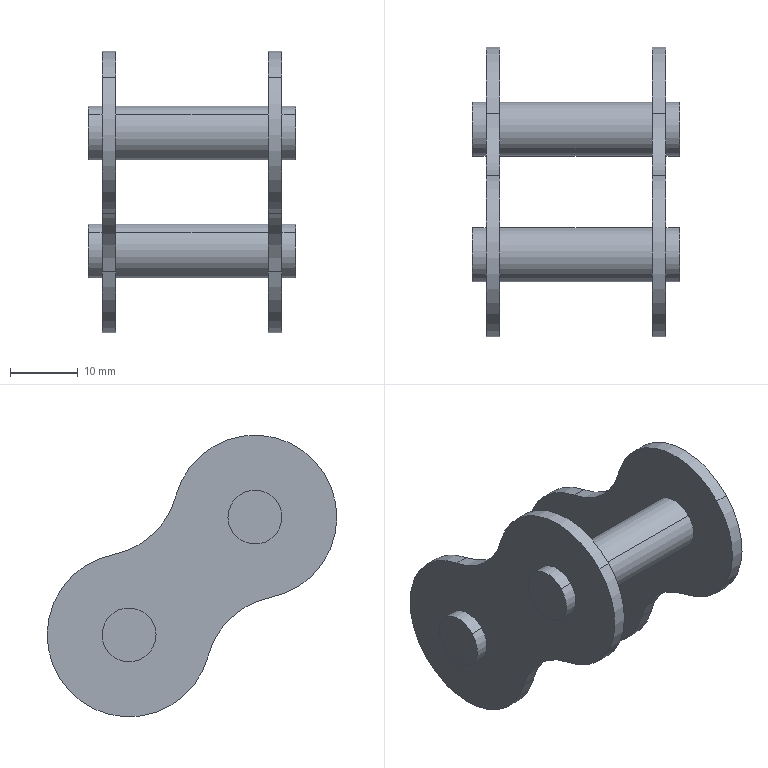Part | STEP file | Mirror 2-38 | 1 solid | 32 faces | box 30.5 x 42.672 x 41.49 mm | volume 6536 mm3 | cylinder 24 | plane 8 | commonest cylinder face diameters 7.94 x12 24.13 x8 23.785 x4
STEP:
#1=CARTESIAN_POINT('',(36.684,-617.915,2791.222));
#2=VERTEX_POINT('',#1);
#3=CARTESIAN_POINT('',(36.684,-624.399,2811.307));
#4=VERTEX_POINT('',#3);
#5=CARTESIAN_POINT('',(36.684,-615.592,2803.061));
#6=DIRECTION('',(-1.,0.,0.));
#7=DIRECTION('',(0.,-0.73,0.6835));
#8=AXIS2_PLACEMENT_3D('',#5,#6,#7);
#9=CIRCLE('',#8,12.065);
#10=EDGE_CURVE('',#2,#4,#9,.T.);
#11=ORIENTED_EDGE('',*,*,#10,.T.);
#12=CARTESIAN_POINT('',(34.684,-624.399,2811.307));
#13=VERTEX_POINT('',#12);
#14=CARTESIAN_POINT('',(36.684,-624.399,2811.307));
#15=DIRECTION('',(-1.,0.,0.));
#16=VECTOR('',#15,1000.);
#17=LINE('',#14,#16);
#18=EDGE_CURVE('',#4,#13,#17,.T.);
#19=ORIENTED_EDGE('',*,*,#18,.T.);
#20=CARTESIAN_POINT('',(34.684,-617.915,2791.222));
#21=VERTEX_POINT('',#20);
#22=CARTESIAN_POINT('',(34.684,-615.592,2803.061));
#23=DIRECTION('',(-1.,0.,0.));
#24=DIRECTION('',(0.,-0.73,0.6835));
#25=AXIS2_PLACEMENT_3D('',#22,#23,#24);
#26=CIRCLE('',#25,12.065);
#27=EDGE_CURVE('',#21,#13,#26,.T.);
#28=ORIENTED_EDGE('',*,*,#27,.F.);
#29=CARTESIAN_POINT('',(36.684,-617.915,2791.222));
#30=DIRECTION('',(-1.,0.,0.));
#31=VECTOR('',#30,1000.);
#32=LINE('',#29,#31);
#33=EDGE_CURVE('',#2,#21,#32,.T.);
#34=ORIENTED_EDGE('',*,*,#33,.F.);
#35=EDGE_LOOP('',(#11,#19,#28,#34));
#36=FACE_OUTER_BOUND('',#35,.T.);
#37=CARTESIAN_POINT('',(36.684,-615.592,2803.061));
#38=DIRECTION('',(-1.,0.,0.));
#39=DIRECTION('',(0.,-0.73,0.6835));
#40=AXIS2_PLACEMENT_3D('',#37,#38,#39);
#41=CYLINDRICAL_SURFACE('',#40,12.065);
#42=ADVANCED_FACE('',(#36),#41,.T.);
#43=CARTESIAN_POINT('',(59.184,-624.399,2811.307));
#44=VERTEX_POINT('',#43);
#45=CARTESIAN_POINT('',(59.184,-603.931,2806.158));
#46=VERTEX_POINT('',#45);
#47=CARTESIAN_POINT('',(59.184,-615.592,2803.061));
#48=DIRECTION('',(-1.,0.,0.));
#49=DIRECTION('',(0.,-0.73,0.6835));
#50=AXIS2_PLACEMENT_3D('',#47,#48,#49);
#51=CIRCLE('',#50,12.065);
#52=EDGE_CURVE('',#44,#46,#51,.T.);
#53=ORIENTED_EDGE('',*,*,#52,.F.);
#54=CARTESIAN_POINT('',(61.184,-624.399,2811.307));
#55=VERTEX_POINT('',#54);
#56=CARTESIAN_POINT('',(59.184,-624.399,2811.307));
#57=DIRECTION('',(1.,0.,0.));
#58=VECTOR('',#57,1000.);
#59=LINE('',#56,#58);
#60=EDGE_CURVE('',#44,#55,#59,.T.);
#61=ORIENTED_EDGE('',*,*,#60,.T.);
#62=CARTESIAN_POINT('',(61.184,-603.931,2806.158));
#63=VERTEX_POINT('',#62);
#64=CARTESIAN_POINT('',(61.184,-615.592,2803.061));
#65=DIRECTION('',(-1.,0.,0.));
#66=DIRECTION('',(0.,-0.73,0.6835));
#67=AXIS2_PLACEMENT_3D('',#64,#65,#66);
#68=CIRCLE('',#67,12.065);
#69=EDGE_CURVE('',#55,#63,#68,.T.);
#70=ORIENTED_EDGE('',*,*,#69,.T.);
#71=CARTESIAN_POINT('',(59.184,-603.931,2806.158));
#72=DIRECTION('',(1.,0.,0.));
#73=VECTOR('',#72,1000.);
#74=LINE('',#71,#73);
#75=EDGE_CURVE('',#46,#63,#74,.T.);
#76=ORIENTED_EDGE('',*,*,#75,.F.);
#77=EDGE_LOOP('',(#53,#61,#70,#76));
#78=FACE_OUTER_BOUND('',#77,.T.);
#79=CARTESIAN_POINT('',(59.184,-615.592,2803.061));
#80=DIRECTION('',(1.,0.,0.));
#81=DIRECTION('',(0.,-0.73,0.6835));
#82=AXIS2_PLACEMENT_3D('',#79,#80,#81);
#83=CYLINDRICAL_SURFACE('',#82,12.065);
#84=ADVANCED_FACE('',(#78),#83,.T.);
#85=CARTESIAN_POINT('',(34.684,-594.152,2782.988));
#86=VERTEX_POINT('',#85);
#87=CARTESIAN_POINT('',(34.684,-599.948,2788.414));
#88=VERTEX_POINT('',#87);
#89=CARTESIAN_POINT('',(34.684,-597.05,2785.701));
#90=DIRECTION('',(-1.,0.,0.));
#91=DIRECTION('',(0.,0.73,-0.6835));
#92=AXIS2_PLACEMENT_3D('',#89,#90,#91);
#93=CIRCLE('',#92,3.97);
#94=EDGE_CURVE('',#86,#88,#93,.T.);
#95=ORIENTED_EDGE('',*,*,#94,.T.);
#96=CARTESIAN_POINT('',(32.684,-599.948,2788.414));
#97=VERTEX_POINT('',#96);
#98=CARTESIAN_POINT('',(47.934,-599.948,2788.414));
#99=DIRECTION('',(1.,0.,0.));
#100=VECTOR('',#99,1000.);
#101=LINE('',#98,#100);
#102=EDGE_CURVE('',#97,#88,#101,.T.);
#103=ORIENTED_EDGE('',*,*,#102,.F.);
#104=CARTESIAN_POINT('',(32.684,-594.152,2782.988));
#105=VERTEX_POINT('',#104);
#106=CARTESIAN_POINT('',(32.684,-597.05,2785.701));
#107=DIRECTION('',(-1.,0.,0.));
#108=DIRECTION('',(0.,-0.73,0.6835));
#109=AXIS2_PLACEMENT_3D('',#106,#107,#108);
#110=CIRCLE('',#109,3.97);
#111=EDGE_CURVE('',#105,#97,#110,.T.);
#112=ORIENTED_EDGE('',*,*,#111,.F.);
#113=CARTESIAN_POINT('',(47.934,-594.152,2782.988));
#114=DIRECTION('',(1.,0.,0.));
#115=VECTOR('',#114,1000.);
#116=LINE('',#113,#115);
#117=EDGE_CURVE('',#105,#86,#116,.T.);
#118=ORIENTED_EDGE('',*,*,#117,.T.);
#119=EDGE_LOOP('',(#95,#103,#112,#118));
#120=FACE_OUTER_BOUND('',#119,.T.);
#121=CARTESIAN_POINT('',(47.934,-597.05,2785.701));
#122=DIRECTION('',(-1.,0.,0.));
#123=DIRECTION('',(0.,-0.73,0.6835));
#124=AXIS2_PLACEMENT_3D('',#121,#122,#123);
#125=CYLINDRICAL_SURFACE('',#124,3.97);
#126=ADVANCED_FACE('',(#120),#125,.T.);
#127=CARTESIAN_POINT('',(34.684,-612.694,2800.348));
#128=VERTEX_POINT('',#127);
#129=CARTESIAN_POINT('',(34.684,-618.49,2805.774));
#130=VERTEX_POINT('',#129);
#131=CARTESIAN_POINT('',(34.684,-615.592,2803.061));
#132=DIRECTION('',(-1.,0.,0.));
#133=DIRECTION('',(0.,0.73,-0.6835));
#134=AXIS2_PLACEMENT_3D('',#131,#132,#133);
#135=CIRCLE('',#134,3.97);
#136=EDGE_CURVE('',#128,#130,#135,.T.);
#137=ORIENTED_EDGE('',*,*,#136,.T.);
#138=CARTESIAN_POINT('',(32.684,-618.49,2805.774));
#139=VERTEX_POINT('',#138);
#140=CARTESIAN_POINT('',(47.934,-618.49,2805.774));
#141=DIRECTION('',(1.,0.,0.));
#142=VECTOR('',#141,1000.);
#143=LINE('',#140,#142);
#144=EDGE_CURVE('',#139,#130,#143,.T.);
#145=ORIENTED_EDGE('',*,*,#144,.F.);
#146=CARTESIAN_POINT('',(32.684,-612.694,2800.348));
#147=VERTEX_POINT('',#146);
#148=CARTESIAN_POINT('',(32.684,-615.592,2803.061));
#149=DIRECTION('',(-1.,0.,0.));
#150=DIRECTION('',(0.,-0.73,0.6835));
#151=AXIS2_PLACEMENT_3D('',#148,#149,#150);
#152=CIRCLE('',#151,3.97);
#153=EDGE_CURVE('',#147,#139,#152,.T.);
#154=ORIENTED_EDGE('',*,*,#153,.F.);
#155=CARTESIAN_POINT('',(47.934,-612.694,2800.348));
#156=DIRECTION('',(1.,0.,0.));
#157=VECTOR('',#156,1000.);
#158=LINE('',#155,#157);
#159=EDGE_CURVE('',#147,#128,#158,.T.);
#160=ORIENTED_EDGE('',*,*,#159,.T.);
#161=EDGE_LOOP('',(#137,#145,#154,#160));
#162=FACE_OUTER_BOUND('',#161,.T.);
#163=CARTESIAN_POINT('',(47.934,-615.592,2803.061));
#164=DIRECTION('',(-1.,0.,0.));
#165=DIRECTION('',(0.,-0.73,0.6835));
#166=AXIS2_PLACEMENT_3D('',#163,#164,#165);
#167=CYLINDRICAL_SURFACE('',#166,3.97);
#168=ADVANCED_FACE('',(#162),#167,.T.);
#169=CARTESIAN_POINT('',(36.684,-594.727,2797.54));
#170=VERTEX_POINT('',#169);
#171=CARTESIAN_POINT('',(36.684,-588.243,2777.455));
#172=VERTEX_POINT('',#171);
#173=CARTESIAN_POINT('',(36.684,-597.05,2785.701));
#174=DIRECTION('',(-1.,0.,0.));
#175=DIRECTION('',(0.,-0.73,0.6835));
#176=AXIS2_PLACEMENT_3D('',#173,#174,#175);
#177=CIRCLE('',#176,12.065);
#178=EDGE_CURVE('',#170,#172,#177,.T.);
#179=ORIENTED_EDGE('',*,*,#178,.T.);
#180=CARTESIAN_POINT('',(34.684,-588.243,2777.455));
#181=VERTEX_POINT('',#180);
#182=CARTESIAN_POINT('',(36.684,-588.243,2777.455));
#183=DIRECTION('',(-1.,0.,0.));
#184=VECTOR('',#183,1000.);
#185=LINE('',#182,#184);
#186=EDGE_CURVE('',#172,#181,#185,.T.);
#187=ORIENTED_EDGE('',*,*,#186,.T.);
#188=CARTESIAN_POINT('',(34.684,-594.727,2797.54));
#189=VERTEX_POINT('',#188);
#190=CARTESIAN_POINT('',(34.684,-597.05,2785.701));
#191=DIRECTION('',(-1.,0.,0.));
#192=DIRECTION('',(0.,-0.73,0.6835));
#193=AXIS2_PLACEMENT_3D('',#190,#191,#192);
#194=CIRCLE('',#193,12.065);
#195=EDGE_CURVE('',#189,#181,#194,.T.);
#196=ORIENTED_EDGE('',*,*,#195,.F.);
#197=CARTESIAN_POINT('',(36.684,-594.727,2797.54));
#198=DIRECTION('',(-1.,0.,0.));
#199=VECTOR('',#198,1000.);
#200=LINE('',#197,#199);
#201=EDGE_CURVE('',#170,#189,#200,.T.);
#202=ORIENTED_EDGE('',*,*,#201,.F.);
#203=EDGE_LOOP('',(#179,#187,#196,#202));
#204=FACE_OUTER_BOUND('',#203,.T.);
#205=CARTESIAN_POINT('',(36.684,-597.05,2785.701));
#206=DIRECTION('',(-1.,0.,0.));
#207=DIRECTION('',(0.,-0.73,0.6835));
#208=AXIS2_PLACEMENT_3D('',#205,#206,#207);
#209=CYLINDRICAL_SURFACE('',#208,12.065);
#210=ADVANCED_FACE('',(#204),#209,.T.);
#211=CARTESIAN_POINT('',(36.684,-599.948,2788.414));
#212=VERTEX_POINT('',#211);
#213=CARTESIAN_POINT('',(36.684,-594.152,2782.988));
#214=VERTEX_POINT('',#213);
#215=CARTESIAN_POINT('',(36.684,-597.05,2785.701));
#216=DIRECTION('',(-1.,0.,0.));
#217=DIRECTION('',(0.,-0.73,0.6835));
#218=AXIS2_PLACEMENT_3D('',#215,#216,#217);
#219=CIRCLE('',#218,3.97);
#220=EDGE_CURVE('',#212,#214,#219,.T.);
#221=ORIENTED_EDGE('',*,*,#220,.F.);
#222=CARTESIAN_POINT('',(59.184,-599.948,2788.414));
#223=VERTEX_POINT('',#222);
#224=CARTESIAN_POINT('',(47.934,-599.948,2788.414));
#225=DIRECTION('',(-1.,0.,0.));
#226=VECTOR('',#225,1000.);
#227=LINE('',#224,#226);
#228=EDGE_CURVE('',#223,#212,#227,.T.);
#229=ORIENTED_EDGE('',*,*,#228,.F.);
#230=CARTESIAN_POINT('',(59.184,-594.152,2782.988));
#231=VERTEX_POINT('',#230);
#232=CARTESIAN_POINT('',(59.184,-597.05,2785.701));
#233=DIRECTION('',(-1.,0.,0.));
#234=DIRECTION('',(0.,-0.73,0.6835));
#235=AXIS2_PLACEMENT_3D('',#232,#233,#234);
#236=CIRCLE('',#235,3.97);
#237=EDGE_CURVE('',#223,#231,#236,.T.);
#238=ORIENTED_EDGE('',*,*,#237,.T.);
#239=CARTESIAN_POINT('',(47.934,-594.152,2782.988));
#240=DIRECTION('',(-1.,0.,0.));
#241=VECTOR('',#240,1000.);
#242=LINE('',#239,#241);
#243=EDGE_CURVE('',#231,#214,#242,.T.);
#244=ORIENTED_EDGE('',*,*,#243,.T.);
#245=EDGE_LOOP('',(#221,#229,#238,#244));
#246=FACE_OUTER_BOUND('',#245,.T.);
#247=CARTESIAN_POINT('',(47.934,-597.05,2785.701));
#248=DIRECTION('',(1.,0.,0.));
#249=DIRECTION('',(0.,-0.73,0.6835));
#250=AXIS2_PLACEMENT_3D('',#247,#248,#249);
#251=CYLINDRICAL_SURFACE('',#250,3.97);
#252=ADVANCED_FACE('',(#246),#251,.T.);
#253=CARTESIAN_POINT('',(61.184,-599.948,2788.414));
#254=VERTEX_POINT('',#253);
#255=CARTESIAN_POINT('',(61.184,-594.152,2782.988));
#256=VERTEX_POINT('',#255);
#257=CARTESIAN_POINT('',(61.184,-597.05,2785.701));
#258=DIRECTION('',(-1.,0.,0.));
#259=DIRECTION('',(0.,0.73,-0.6835));
#260=AXIS2_PLACEMENT_3D('',#257,#258,#259);
#261=CIRCLE('',#260,3.97);
#262=EDGE_CURVE('',#254,#256,#261,.T.);
#263=ORIENTED_EDGE('',*,*,#262,.F.);
#264=CARTESIAN_POINT('',(63.184,-599.948,2788.414));
#265=VERTEX_POINT('',#264);
#266=CARTESIAN_POINT('',(47.934,-599.948,2788.414));
#267=DIRECTION('',(-1.,0.,0.));
#268=VECTOR('',#267,1000.);
#269=LINE('',#266,#268);
#270=EDGE_CURVE('',#265,#254,#269,.T.);
#271=ORIENTED_EDGE('',*,*,#270,.F.);
#272=CARTESIAN_POINT('',(63.184,-594.152,2782.988));
#273=VERTEX_POINT('',#272);
#274=CARTESIAN_POINT('',(63.184,-597.05,2785.701));
#275=DIRECTION('',(-1.,0.,0.));
#276=DIRECTION('',(0.,-0.73,0.6835));
#277=AXIS2_PLACEMENT_3D('',#274,#275,#276);
#278=CIRCLE('',#277,3.97);
#279=EDGE_CURVE('',#265,#273,#278,.T.);
#280=ORIENTED_EDGE('',*,*,#279,.T.);
#281=CARTESIAN_POINT('',(47.934,-594.152,2782.988));
#282=DIRECTION('',(-1.,0.,0.));
#283=VECTOR('',#282,1000.);
#284=LINE('',#281,#283);
#285=EDGE_CURVE('',#273,#256,#284,.T.);
#286=ORIENTED_EDGE('',*,*,#285,.T.);
#287=EDGE_LOOP('',(#263,#271,#280,#286));
#288=FACE_OUTER_BOUND('',#287,.T.);
#289=CARTESIAN_POINT('',(47.934,-597.05,2785.701));
#290=DIRECTION('',(1.,0.,0.));
#291=DIRECTION('',(0.,-0.73,0.6835));
#292=AXIS2_PLACEMENT_3D('',#289,#290,#291);
#293=CYLINDRICAL_SURFACE('',#292,3.97);
#294=ADVANCED_FACE('',(#288),#293,.T.);
#295=CARTESIAN_POINT('',(36.684,-618.49,2805.774));
#296=VERTEX_POINT('',#295);
#297=CARTESIAN_POINT('',(36.684,-612.694,2800.348));
#298=VERTEX_POINT('',#297);
#299=CARTESIAN_POINT('',(36.684,-615.592,2803.061));
#300=DIRECTION('',(-1.,0.,0.));
#301=DIRECTION('',(0.,-0.73,0.6835));
#302=AXIS2_PLACEMENT_3D('',#299,#300,#301);
#303=CIRCLE('',#302,3.97);
#304=EDGE_CURVE('',#296,#298,#303,.T.);
#305=ORIENTED_EDGE('',*,*,#304,.F.);
#306=CARTESIAN_POINT('',(59.184,-618.49,2805.774));
#307=VERTEX_POINT('',#306);
#308=CARTESIAN_POINT('',(47.934,-618.49,2805.774));
#309=DIRECTION('',(-1.,0.,0.));
#310=VECTOR('',#309,1000.);
#311=LINE('',#308,#310);
#312=EDGE_CURVE('',#307,#296,#311,.T.);
#313=ORIENTED_EDGE('',*,*,#312,.F.);
#314=CARTESIAN_POINT('',(59.184,-612.694,2800.348));
#315=VERTEX_POINT('',#314);
#316=CARTESIAN_POINT('',(59.184,-615.592,2803.061));
#317=DIRECTION('',(-1.,0.,0.));
#318=DIRECTION('',(0.,-0.73,0.6835));
#319=AXIS2_PLACEMENT_3D('',#316,#317,#318);
#320=CIRCLE('',#319,3.97);
#321=EDGE_CURVE('',#307,#315,#320,.T.);
#322=ORIENTED_EDGE('',*,*,#321,.T.);
#323=CARTESIAN_POINT('',(47.934,-612.694,2800.348));
#324=DIRECTION('',(-1.,0.,0.));
#325=VECTOR('',#324,1000.);
#326=LINE('',#323,#325);
#327=EDGE_CURVE('',#315,#298,#326,.T.);
#328=ORIENTED_EDGE('',*,*,#327,.T.);
#329=EDGE_LOOP('',(#305,#313,#322,#328));
#330=FACE_OUTER_BOUND('',#329,.T.);
#331=CARTESIAN_POINT('',(47.934,-615.592,2803.061));
#332=DIRECTION('',(1.,0.,0.));
#333=DIRECTION('',(0.,-0.73,0.6835));
#334=AXIS2_PLACEMENT_3D('',#331,#332,#333);
#335=CYLINDRICAL_SURFACE('',#334,3.97);
#336=ADVANCED_FACE('',(#330),#335,.T.);
#337=CARTESIAN_POINT('',(61.184,-618.49,2805.774));
#338=VERTEX_POINT('',#337);
#339=CARTESIAN_POINT('',(61.184,-612.694,2800.348));
#340=VERTEX_POINT('',#339);
#341=CARTESIAN_POINT('',(61.184,-615.592,2803.061));
#342=DIRECTION('',(-1.,0.,0.));
#343=DIRECTION('',(0.,0.73,-0.6835));
#344=AXIS2_PLACEMENT_3D('',#341,#342,#343);
#345=CIRCLE('',#344,3.97);
#346=EDGE_CURVE('',#338,#340,#345,.T.);
#347=ORIENTED_EDGE('',*,*,#346,.F.);
#348=CARTESIAN_POINT('',(63.184,-618.49,2805.774));
#349=VERTEX_POINT('',#348);
#350=CARTESIAN_POINT('',(47.934,-618.49,2805.774));
#351=DIRECTION('',(-1.,0.,0.));
#352=VECTOR('',#351,1000.);
#353=LINE('',#350,#352);
#354=EDGE_CURVE('',#349,#338,#353,.T.);
#355=ORIENTED_EDGE('',*,*,#354,.F.);
#356=CARTESIAN_POINT('',(63.184,-612.694,2800.348));
#357=VERTEX_POINT('',#356);
#358=CARTESIAN_POINT('',(63.184,-615.592,2803.061));
#359=DIRECTION('',(-1.,0.,0.));
#360=DIRECTION('',(0.,-0.73,0.6835));
#361=AXIS2_PLACEMENT_3D('',#358,#359,#360);
#362=CIRCLE('',#361,3.97);
#363=EDGE_CURVE('',#349,#357,#362,.T.);
#364=ORIENTED_EDGE('',*,*,#363,.T.);
#365=CARTESIAN_POINT('',(47.934,-612.694,2800.348));
#366=DIRECTION('',(-1.,0.,0.));
#367=VECTOR('',#366,1000.);
#368=LINE('',#365,#367);
#369=EDGE_CURVE('',#357,#340,#368,.T.);
#370=ORIENTED_EDGE('',*,*,#369,.T.);
#371=EDGE_LOOP('',(#347,#355,#364,#370));
#372=FACE_OUTER_BOUND('',#371,.T.);
#373=CARTESIAN_POINT('',(47.934,-615.592,2803.061));
#374=DIRECTION('',(1.,0.,0.));
#375=DIRECTION('',(0.,-0.73,0.6835));
#376=AXIS2_PLACEMENT_3D('',#373,#374,#375);
#377=CYLINDRICAL_SURFACE('',#376,3.97);
#378=ADVANCED_FACE('',(#372),#377,.T.);
#379=CARTESIAN_POINT('',(59.184,-588.243,2777.455));
#380=VERTEX_POINT('',#379);
#381=CARTESIAN_POINT('',(59.184,-608.711,2782.604));
#382=VERTEX_POINT('',#381);
#383=CARTESIAN_POINT('',(59.184,-597.05,2785.701));
#384=DIRECTION('',(-1.,0.,0.));
#385=DIRECTION('',(0.,-0.73,0.6835));
#386=AXIS2_PLACEMENT_3D('',#383,#384,#385);
#387=CIRCLE('',#386,12.065);
#388=EDGE_CURVE('',#380,#382,#387,.T.);
#389=ORIENTED_EDGE('',*,*,#388,.F.);
#390=CARTESIAN_POINT('',(61.184,-588.243,2777.455));
#391=VERTEX_POINT('',#390);
#392=CARTESIAN_POINT('',(59.184,-588.243,2777.455));
#393=DIRECTION('',(1.,0.,0.));
#394=VECTOR('',#393,1000.);
#395=LINE('',#392,#394);
#396=EDGE_CURVE('',#380,#391,#395,.T.);
#397=ORIENTED_EDGE('',*,*,#396,.T.);
#398=CARTESIAN_POINT('',(61.184,-608.711,2782.604));
#399=VERTEX_POINT('',#398);
#400=CARTESIAN_POINT('',(61.184,-597.05,2785.701));
#401=DIRECTION('',(-1.,0.,0.));
#402=DIRECTION('',(0.,-0.73,0.6835));
#403=AXIS2_PLACEMENT_3D('',#400,#401,#402);
#404=CIRCLE('',#403,12.065);
#405=EDGE_CURVE('',#391,#399,#404,.T.);
#406=ORIENTED_EDGE('',*,*,#405,.T.);
#407=CARTESIAN_POINT('',(59.184,-608.711,2782.604));
#408=DIRECTION('',(1.,0.,0.));
#409=VECTOR('',#408,1000.);
#410=LINE('',#407,#409);
#411=EDGE_CURVE('',#382,#399,#410,.T.);
#412=ORIENTED_EDGE('',*,*,#411,.F.);
#413=EDGE_LOOP('',(#389,#397,#406,#412));
#414=FACE_OUTER_BOUND('',#413,.T.);
#415=CARTESIAN_POINT('',(59.184,-597.05,2785.701));
#416=DIRECTION('',(1.,0.,0.));
#417=DIRECTION('',(0.,-0.73,0.6835));
#418=AXIS2_PLACEMENT_3D('',#415,#416,#417);
#419=CYLINDRICAL_SURFACE('',#418,12.065);
#420=ADVANCED_FACE('',(#414),#419,.T.);
#421=CARTESIAN_POINT('',(59.184,-594.727,2797.54));
#422=VERTEX_POINT('',#421);
#423=CARTESIAN_POINT('',(59.184,-592.437,2809.21));
#424=DIRECTION('',(1.,0.,0.));
#425=DIRECTION('',(0.,0.73,-0.6835));
#426=AXIS2_PLACEMENT_3D('',#423,#424,#425);
#427=CIRCLE('',#426,11.892);
#428=EDGE_CURVE('',#46,#422,#427,.T.);
#429=ORIENTED_EDGE('',*,*,#428,.T.);
#430=CARTESIAN_POINT('',(59.184,-597.05,2785.701));
#431=DIRECTION('',(-1.,0.,0.));
#432=DIRECTION('',(0.,-0.73,0.6835));
#433=AXIS2_PLACEMENT_3D('',#430,#431,#432);
#434=CIRCLE('',#433,12.065);
#435=EDGE_CURVE('',#422,#380,#434,.T.);
#436=ORIENTED_EDGE('',*,*,#435,.T.);
#437=ORIENTED_EDGE('',*,*,#388,.T.);
#438=CARTESIAN_POINT('',(59.184,-617.915,2791.222));
#439=VERTEX_POINT('',#438);
#440=CARTESIAN_POINT('',(59.184,-620.205,2779.552));
#441=DIRECTION('',(1.,0.,0.));
#442=DIRECTION('',(0.,-0.73,0.6835));
#443=AXIS2_PLACEMENT_3D('',#440,#441,#442);
#444=CIRCLE('',#443,11.892);
#445=EDGE_CURVE('',#382,#439,#444,.T.);
#446=ORIENTED_EDGE('',*,*,#445,.T.);
#447=CARTESIAN_POINT('',(59.184,-615.592,2803.061));
#448=DIRECTION('',(-1.,0.,0.));
#449=DIRECTION('',(0.,-0.73,0.6835));
#450=AXIS2_PLACEMENT_3D('',#447,#448,#449);
#451=CIRCLE('',#450,12.065);
#452=EDGE_CURVE('',#439,#44,#451,.T.);
#453=ORIENTED_EDGE('',*,*,#452,.T.);
#454=ORIENTED_EDGE('',*,*,#52,.T.);
#455=EDGE_LOOP('',(#429,#436,#437,#446,#453,#454));
#456=FACE_OUTER_BOUND('',#455,.T.);
#457=CARTESIAN_POINT('',(59.184,-615.592,2803.061));
#458=DIRECTION('',(-1.,0.,0.));
#459=DIRECTION('',(0.,-0.73,0.6835));
#460=AXIS2_PLACEMENT_3D('',#457,#458,#459);
#461=CIRCLE('',#460,3.97);
#462=EDGE_CURVE('',#315,#307,#461,.T.);
#463=ORIENTED_EDGE('',*,*,#462,.F.);
#464=ORIENTED_EDGE('',*,*,#321,.F.);
#465=EDGE_LOOP('',(#463,#464));
#466=FACE_BOUND('',#465,.T.);
#467=CARTESIAN_POINT('',(59.184,-597.05,2785.701));
#468=DIRECTION('',(-1.,0.,0.));
#469=DIRECTION('',(0.,-0.73,0.6835));
#470=AXIS2_PLACEMENT_3D('',#467,#468,#469);
#471=CIRCLE('',#470,3.97);
#472=EDGE_CURVE('',#231,#223,#471,.T.);
#473=ORIENTED_EDGE('',*,*,#472,.F.);
#474=ORIENTED_EDGE('',*,*,#237,.F.);
#475=EDGE_LOOP('',(#473,#474));
#476=FACE_BOUND('',#475,.T.);
#477=CARTESIAN_POINT('',(59.184,-594.743,2797.456));
#478=DIRECTION('',(1.,0.,0.));
#479=DIRECTION('',(0.,-0.73,0.6835));
#480=AXIS2_PLACEMENT_3D('',#477,#478,#479);
#481=PLANE('',#480);
#482=ADVANCED_FACE('',(#456,#466,#476),#481,.F.);
#483=CARTESIAN_POINT('',(61.184,-615.592,2803.061));
#484=DIRECTION('',(-1.,0.,0.));
#485=DIRECTION('',(0.,0.73,-0.6835));
#486=AXIS2_PLACEMENT_3D('',#483,#484,#485);
#487=CIRCLE('',#486,3.97);
#488=EDGE_CURVE('',#340,#338,#487,.T.);
#489=ORIENTED_EDGE('',*,*,#488,.T.);
#490=ORIENTED_EDGE('',*,*,#346,.T.);
#491=EDGE_LOOP('',(#489,#490));
#492=FACE_BOUND('',#491,.T.);
#493=CARTESIAN_POINT('',(61.184,-594.727,2797.54));
#494=VERTEX_POINT('',#493);
#495=CARTESIAN_POINT('',(61.184,-592.437,2809.21));
#496=DIRECTION('',(1.,0.,0.));
#497=DIRECTION('',(0.,0.73,-0.6835));
#498=AXIS2_PLACEMENT_3D('',#495,#496,#497);
#499=CIRCLE('',#498,11.892);
#500=EDGE_CURVE('',#63,#494,#499,.T.);
#501=ORIENTED_EDGE('',*,*,#500,.F.);
#502=ORIENTED_EDGE('',*,*,#69,.F.);
#503=CARTESIAN_POINT('',(61.184,-617.915,2791.222));
#504=VERTEX_POINT('',#503);
#505=CARTESIAN_POINT('',(61.184,-615.592,2803.061));
#506=DIRECTION('',(-1.,0.,0.));
#507=DIRECTION('',(0.,-0.73,0.6835));
#508=AXIS2_PLACEMENT_3D('',#505,#506,#507);
#509=CIRCLE('',#508,12.065);
#510=EDGE_CURVE('',#504,#55,#509,.T.);
#511=ORIENTED_EDGE('',*,*,#510,.F.);
#512=CARTESIAN_POINT('',(61.184,-620.205,2779.552));
#513=DIRECTION('',(1.,0.,0.));
#514=DIRECTION('',(0.,-0.73,0.6835));
#515=AXIS2_PLACEMENT_3D('',#512,#513,#514);
#516=CIRCLE('',#515,11.892);
#517=EDGE_CURVE('',#399,#504,#516,.T.);
#518=ORIENTED_EDGE('',*,*,#517,.F.);
#519=ORIENTED_EDGE('',*,*,#405,.F.);
#520=CARTESIAN_POINT('',(61.184,-597.05,2785.701));
#521=DIRECTION('',(-1.,0.,0.));
#522=DIRECTION('',(0.,-0.73,0.6835));
#523=AXIS2_PLACEMENT_3D('',#520,#521,#522);
#524=CIRCLE('',#523,12.065);
#525=EDGE_CURVE('',#494,#391,#524,.T.);
#526=ORIENTED_EDGE('',*,*,#525,.F.);
#527=EDGE_LOOP('',(#501,#502,#511,#518,#519,#526));
#528=FACE_OUTER_BOUND('',#527,.T.);
#529=CARTESIAN_POINT('',(61.184,-597.05,2785.701));
#530=DIRECTION('',(-1.,0.,0.));
#531=DIRECTION('',(0.,0.73,-0.6835));
#532=AXIS2_PLACEMENT_3D('',#529,#530,#531);
#533=CIRCLE('',#532,3.97);
#534=EDGE_CURVE('',#256,#254,#533,.T.);
#535=ORIENTED_EDGE('',*,*,#534,.T.);
#536=ORIENTED_EDGE('',*,*,#262,.T.);
#537=EDGE_LOOP('',(#535,#536));
#538=FACE_BOUND('',#537,.T.);
#539=CARTESIAN_POINT('',(61.184,-594.743,2797.456));
#540=DIRECTION('',(1.,0.,0.));
#541=DIRECTION('',(0.,-0.73,0.6835));
#542=AXIS2_PLACEMENT_3D('',#539,#540,#541);
#543=PLANE('',#542);
#544=ADVANCED_FACE('',(#492,#528,#538),#543,.T.);
#545=ORIENTED_EDGE('',*,*,#500,.T.);
#546=CARTESIAN_POINT('',(59.184,-594.727,2797.54));
#547=DIRECTION('',(1.,0.,0.));
#548=VECTOR('',#547,1000.);
#549=LINE('',#546,#548);
#550=EDGE_CURVE('',#422,#494,#549,.T.);
#551=ORIENTED_EDGE('',*,*,#550,.F.);
#552=ORIENTED_EDGE('',*,*,#428,.F.);
#553=ORIENTED_EDGE('',*,*,#75,.T.);
#554=EDGE_LOOP('',(#545,#551,#552,#553));
#555=FACE_OUTER_BOUND('',#554,.T.);
#556=CARTESIAN_POINT('',(59.184,-592.437,2809.21));
#557=DIRECTION('',(1.,0.,0.));
#558=DIRECTION('',(0.,-0.73,0.6835));
#559=AXIS2_PLACEMENT_3D('',#556,#557,#558);
#560=CYLINDRICAL_SURFACE('',#559,11.892);
#561=ADVANCED_FACE('',(#555),#560,.F.);
#562=ORIENTED_EDGE('',*,*,#396,.F.);
#563=ORIENTED_EDGE('',*,*,#435,.F.);
#564=ORIENTED_EDGE('',*,*,#550,.T.);
#565=ORIENTED_EDGE('',*,*,#525,.T.);
#566=EDGE_LOOP('',(#562,#563,#564,#565));
#567=FACE_OUTER_BOUND('',#566,.T.);
#568=CARTESIAN_POINT('',(59.184,-597.05,2785.701));
#569=DIRECTION('',(1.,0.,0.));
#570=DIRECTION('',(0.,-0.73,0.6835));
#571=AXIS2_PLACEMENT_3D('',#568,#569,#570);
#572=CYLINDRICAL_SURFACE('',#571,12.065);
#573=ADVANCED_FACE('',(#567),#572,.T.);
#574=ORIENTED_EDGE('',*,*,#517,.T.);
#575=CARTESIAN_POINT('',(59.184,-617.915,2791.222));
#576=DIRECTION('',(1.,0.,0.));
#577=VECTOR('',#576,1000.);
#578=LINE('',#575,#577);
#579=EDGE_CURVE('',#439,#504,#578,.T.);
#580=ORIENTED_EDGE('',*,*,#579,.F.);
#581=ORIENTED_EDGE('',*,*,#445,.F.);
#582=ORIENTED_EDGE('',*,*,#411,.T.);
#583=EDGE_LOOP('',(#574,#580,#581,#582));
#584=FACE_OUTER_BOUND('',#583,.T.);
#585=CARTESIAN_POINT('',(59.184,-620.205,2779.552));
#586=DIRECTION('',(1.,0.,0.));
#587=DIRECTION('',(0.,-0.73,0.6835));
#588=AXIS2_PLACEMENT_3D('',#585,#586,#587);
#589=CYLINDRICAL_SURFACE('',#588,11.892);
#590=ADVANCED_FACE('',(#584),#589,.F.);
#591=ORIENTED_EDGE('',*,*,#60,.F.);
#592=ORIENTED_EDGE('',*,*,#452,.F.);
#593=ORIENTED_EDGE('',*,*,#579,.T.);
#594=ORIENTED_EDGE('',*,*,#510,.T.);
#595=EDGE_LOOP('',(#591,#592,#593,#594));
#596=FACE_OUTER_BOUND('',#595,.T.);
#597=CARTESIAN_POINT('',(59.184,-615.592,2803.061));
#598=DIRECTION('',(1.,0.,0.));
#599=DIRECTION('',(0.,-0.73,0.6835));
#600=AXIS2_PLACEMENT_3D('',#597,#598,#599);
#601=CYLINDRICAL_SURFACE('',#600,12.065);
#602=ADVANCED_FACE('',(#596),#601,.T.);
#603=CARTESIAN_POINT('',(63.184,-615.592,2803.061));
#604=DIRECTION('',(-1.,0.,0.));
#605=DIRECTION('',(0.,-0.73,0.6835));
#606=AXIS2_PLACEMENT_3D('',#603,#604,#605);
#607=CIRCLE('',#606,3.97);
#608=EDGE_CURVE('',#357,#349,#607,.T.);
#609=ORIENTED_EDGE('',*,*,#608,.F.);
#610=ORIENTED_EDGE('',*,*,#363,.F.);
#611=EDGE_LOOP('',(#609,#610));
#612=FACE_OUTER_BOUND('',#611,.T.);
#613=CARTESIAN_POINT('',(63.184,-615.592,2803.061));
#614=DIRECTION('',(-1.,0.,0.));
#615=DIRECTION('',(0.,0.73,-0.6835));
#616=AXIS2_PLACEMENT_3D('',#613,#614,#615);
#617=PLANE('',#616);
#618=ADVANCED_FACE('',(#612),#617,.F.);
#619=ORIENTED_EDGE('',*,*,#354,.T.);
#620=ORIENTED_EDGE('',*,*,#488,.F.);
#621=ORIENTED_EDGE('',*,*,#369,.F.);
#622=ORIENTED_EDGE('',*,*,#608,.T.);
#623=EDGE_LOOP('',(#619,#620,#621,#622));
#624=FACE_OUTER_BOUND('',#623,.T.);
#625=CARTESIAN_POINT('',(47.934,-615.592,2803.061));
#626=DIRECTION('',(1.,0.,0.));
#627=DIRECTION('',(0.,-0.73,0.6835));
#628=AXIS2_PLACEMENT_3D('',#625,#626,#627);
#629=CYLINDRICAL_SURFACE('',#628,3.97);
#630=ADVANCED_FACE('',(#624),#629,.T.);
#631=ORIENTED_EDGE('',*,*,#312,.T.);
#632=CARTESIAN_POINT('',(36.684,-615.592,2803.061));
#633=DIRECTION('',(-1.,0.,0.));
#634=DIRECTION('',(0.,-0.73,0.6835));
#635=AXIS2_PLACEMENT_3D('',#632,#633,#634);
#636=CIRCLE('',#635,3.97);
#637=EDGE_CURVE('',#298,#296,#636,.T.);
#638=ORIENTED_EDGE('',*,*,#637,.F.);
#639=ORIENTED_EDGE('',*,*,#327,.F.);
#640=ORIENTED_EDGE('',*,*,#462,.T.);
#641=EDGE_LOOP('',(#631,#638,#639,#640));
#642=FACE_OUTER_BOUND('',#641,.T.);
#643=CARTESIAN_POINT('',(47.934,-615.592,2803.061));
#644=DIRECTION('',(1.,0.,0.));
#645=DIRECTION('',(0.,-0.73,0.6835));
#646=AXIS2_PLACEMENT_3D('',#643,#644,#645);
#647=CYLINDRICAL_SURFACE('',#646,3.97);
#648=ADVANCED_FACE('',(#642),#647,.T.);
#649=CARTESIAN_POINT('',(63.184,-597.05,2785.701));
#650=DIRECTION('',(-1.,0.,0.));
#651=DIRECTION('',(0.,-0.73,0.6835));
#652=AXIS2_PLACEMENT_3D('',#649,#650,#651);
#653=CIRCLE('',#652,3.97);
#654=EDGE_CURVE('',#273,#265,#653,.T.);
#655=ORIENTED_EDGE('',*,*,#654,.F.);
#656=ORIENTED_EDGE('',*,*,#279,.F.);
#657=EDGE_LOOP('',(#655,#656));
#658=FACE_OUTER_BOUND('',#657,.T.);
#659=CARTESIAN_POINT('',(63.184,-597.05,2785.701));
#660=DIRECTION('',(-1.,0.,0.));
#661=DIRECTION('',(0.,0.73,-0.6835));
#662=AXIS2_PLACEMENT_3D('',#659,#660,#661);
#663=PLANE('',#662);
#664=ADVANCED_FACE('',(#658),#663,.F.);
#665=ORIENTED_EDGE('',*,*,#270,.T.);
#666=ORIENTED_EDGE('',*,*,#534,.F.);
#667=ORIENTED_EDGE('',*,*,#285,.F.);
#668=ORIENTED_EDGE('',*,*,#654,.T.);
#669=EDGE_LOOP('',(#665,#666,#667,#668));
#670=FACE_OUTER_BOUND('',#669,.T.);
#671=CARTESIAN_POINT('',(47.934,-597.05,2785.701));
#672=DIRECTION('',(1.,0.,0.));
#673=DIRECTION('',(0.,-0.73,0.6835));
#674=AXIS2_PLACEMENT_3D('',#671,#672,#673);
#675=CYLINDRICAL_SURFACE('',#674,3.97);
#676=ADVANCED_FACE('',(#670),#675,.T.);
#677=ORIENTED_EDGE('',*,*,#228,.T.);
#678=CARTESIAN_POINT('',(36.684,-597.05,2785.701));
#679=DIRECTION('',(-1.,0.,0.));
#680=DIRECTION('',(0.,-0.73,0.6835));
#681=AXIS2_PLACEMENT_3D('',#678,#679,#680);
#682=CIRCLE('',#681,3.97);
#683=EDGE_CURVE('',#214,#212,#682,.T.);
#684=ORIENTED_EDGE('',*,*,#683,.F.);
#685=ORIENTED_EDGE('',*,*,#243,.F.);
#686=ORIENTED_EDGE('',*,*,#472,.T.);
#687=EDGE_LOOP('',(#677,#684,#685,#686));
#688=FACE_OUTER_BOUND('',#687,.T.);
#689=CARTESIAN_POINT('',(47.934,-597.05,2785.701));
#690=DIRECTION('',(1.,0.,0.));
#691=DIRECTION('',(0.,-0.73,0.6835));
#692=AXIS2_PLACEMENT_3D('',#689,#690,#691);
#693=CYLINDRICAL_SURFACE('',#692,3.97);
#694=ADVANCED_FACE('',(#688),#693,.T.);
#695=CARTESIAN_POINT('',(36.684,-603.931,2806.158));
#696=VERTEX_POINT('',#695);
#697=CARTESIAN_POINT('',(36.684,-592.437,2809.21));
#698=DIRECTION('',(1.,0.,0.));
#699=DIRECTION('',(0.,0.73,-0.6835));
#700=AXIS2_PLACEMENT_3D('',#697,#698,#699);
#701=CIRCLE('',#700,11.892);
#702=EDGE_CURVE('',#696,#170,#701,.T.);
#703=ORIENTED_EDGE('',*,*,#702,.F.);
#704=CARTESIAN_POINT('',(36.684,-615.592,2803.061));
#705=DIRECTION('',(-1.,0.,0.));
#706=DIRECTION('',(0.,-0.73,0.6835));
#707=AXIS2_PLACEMENT_3D('',#704,#705,#706);
#708=CIRCLE('',#707,12.065);
#709=EDGE_CURVE('',#4,#696,#708,.T.);
#710=ORIENTED_EDGE('',*,*,#709,.F.);
#711=ORIENTED_EDGE('',*,*,#10,.F.);
#712=CARTESIAN_POINT('',(36.684,-608.711,2782.604));
#713=VERTEX_POINT('',#712);
#714=CARTESIAN_POINT('',(36.684,-620.205,2779.552));
#715=DIRECTION('',(1.,0.,0.));
#716=DIRECTION('',(0.,-0.73,0.6835));
#717=AXIS2_PLACEMENT_3D('',#714,#715,#716);
#718=CIRCLE('',#717,11.892);
#719=EDGE_CURVE('',#713,#2,#718,.T.);
#720=ORIENTED_EDGE('',*,*,#719,.F.);
#721=CARTESIAN_POINT('',(36.684,-597.05,2785.701));
#722=DIRECTION('',(-1.,0.,0.));
#723=DIRECTION('',(0.,-0.73,0.6835));
#724=AXIS2_PLACEMENT_3D('',#721,#722,#723);
#725=CIRCLE('',#724,12.065);
#726=EDGE_CURVE('',#172,#713,#725,.T.);
#727=ORIENTED_EDGE('',*,*,#726,.F.);
#728=ORIENTED_EDGE('',*,*,#178,.F.);
#729=EDGE_LOOP('',(#703,#710,#711,#720,#727,#728));
#730=FACE_OUTER_BOUND('',#729,.T.);
#731=ORIENTED_EDGE('',*,*,#637,.T.);
#732=ORIENTED_EDGE('',*,*,#304,.T.);
#733=EDGE_LOOP('',(#731,#732));
#734=FACE_BOUND('',#733,.T.);
#735=ORIENTED_EDGE('',*,*,#683,.T.);
#736=ORIENTED_EDGE('',*,*,#220,.T.);
#737=EDGE_LOOP('',(#735,#736));
#738=FACE_BOUND('',#737,.T.);
#739=CARTESIAN_POINT('',(36.684,-594.743,2797.456));
#740=DIRECTION('',(-1.,0.,0.));
#741=DIRECTION('',(0.,-0.73,0.6835));
#742=AXIS2_PLACEMENT_3D('',#739,#740,#741);
#743=PLANE('',#742);
#744=ADVANCED_FACE('',(#730,#734,#738),#743,.F.);
#745=ORIENTED_EDGE('',*,*,#136,.F.);
#746=CARTESIAN_POINT('',(34.684,-615.592,2803.061));
#747=DIRECTION('',(-1.,0.,0.));
#748=DIRECTION('',(0.,0.73,-0.6835));
#749=AXIS2_PLACEMENT_3D('',#746,#747,#748);
#750=CIRCLE('',#749,3.97);
#751=EDGE_CURVE('',#130,#128,#750,.T.);
#752=ORIENTED_EDGE('',*,*,#751,.F.);
#753=EDGE_LOOP('',(#745,#752));
#754=FACE_BOUND('',#753,.T.);
#755=CARTESIAN_POINT('',(34.684,-603.931,2806.158));
#756=VERTEX_POINT('',#755);
#757=CARTESIAN_POINT('',(34.684,-592.437,2809.21));
#758=DIRECTION('',(1.,0.,0.));
#759=DIRECTION('',(0.,0.73,-0.6835));
#760=AXIS2_PLACEMENT_3D('',#757,#758,#759);
#761=CIRCLE('',#760,11.892);
#762=EDGE_CURVE('',#756,#189,#761,.T.);
#763=ORIENTED_EDGE('',*,*,#762,.T.);
#764=ORIENTED_EDGE('',*,*,#195,.T.);
#765=CARTESIAN_POINT('',(34.684,-608.711,2782.604));
#766=VERTEX_POINT('',#765);
#767=CARTESIAN_POINT('',(34.684,-597.05,2785.701));
#768=DIRECTION('',(-1.,0.,0.));
#769=DIRECTION('',(0.,-0.73,0.6835));
#770=AXIS2_PLACEMENT_3D('',#767,#768,#769);
#771=CIRCLE('',#770,12.065);
#772=EDGE_CURVE('',#181,#766,#771,.T.);
#773=ORIENTED_EDGE('',*,*,#772,.T.);
#774=CARTESIAN_POINT('',(34.684,-620.205,2779.552));
#775=DIRECTION('',(1.,0.,0.));
#776=DIRECTION('',(0.,-0.73,0.6835));
#777=AXIS2_PLACEMENT_3D('',#774,#775,#776);
#778=CIRCLE('',#777,11.892);
#779=EDGE_CURVE('',#766,#21,#778,.T.);
#780=ORIENTED_EDGE('',*,*,#779,.T.);
#781=ORIENTED_EDGE('',*,*,#27,.T.);
#782=CARTESIAN_POINT('',(34.684,-615.592,2803.061));
#783=DIRECTION('',(-1.,0.,0.));
#784=DIRECTION('',(0.,-0.73,0.6835));
#785=AXIS2_PLACEMENT_3D('',#782,#783,#784);
#786=CIRCLE('',#785,12.065);
#787=EDGE_CURVE('',#13,#756,#786,.T.);
#788=ORIENTED_EDGE('',*,*,#787,.T.);
#789=EDGE_LOOP('',(#763,#764,#773,#780,#781,#788));
#790=FACE_OUTER_BOUND('',#789,.T.);
#791=ORIENTED_EDGE('',*,*,#94,.F.);
#792=CARTESIAN_POINT('',(34.684,-597.05,2785.701));
#793=DIRECTION('',(-1.,0.,0.));
#794=DIRECTION('',(0.,0.73,-0.6835));
#795=AXIS2_PLACEMENT_3D('',#792,#793,#794);
#796=CIRCLE('',#795,3.97);
#797=EDGE_CURVE('',#88,#86,#796,.T.);
#798=ORIENTED_EDGE('',*,*,#797,.F.);
#799=EDGE_LOOP('',(#791,#798));
#800=FACE_BOUND('',#799,.T.);
#801=CARTESIAN_POINT('',(34.684,-594.743,2797.456));
#802=DIRECTION('',(-1.,0.,0.));
#803=DIRECTION('',(0.,-0.73,0.6835));
#804=AXIS2_PLACEMENT_3D('',#801,#802,#803);
#805=PLANE('',#804);
#806=ADVANCED_FACE('',(#754,#790,#800),#805,.T.);
#807=ORIENTED_EDGE('',*,*,#762,.F.);
#808=CARTESIAN_POINT('',(36.684,-603.931,2806.158));
#809=DIRECTION('',(-1.,0.,0.));
#810=VECTOR('',#809,1000.);
#811=LINE('',#808,#810);
#812=EDGE_CURVE('',#696,#756,#811,.T.);
#813=ORIENTED_EDGE('',*,*,#812,.F.);
#814=ORIENTED_EDGE('',*,*,#702,.T.);
#815=ORIENTED_EDGE('',*,*,#201,.T.);
#816=EDGE_LOOP('',(#807,#813,#814,#815));
#817=FACE_OUTER_BOUND('',#816,.T.);
#818=CARTESIAN_POINT('',(36.684,-592.437,2809.21));
#819=DIRECTION('',(-1.,0.,0.));
#820=DIRECTION('',(0.,-0.73,0.6835));
#821=AXIS2_PLACEMENT_3D('',#818,#819,#820);
#822=CYLINDRICAL_SURFACE('',#821,11.892);
#823=ADVANCED_FACE('',(#817),#822,.F.);
#824=ORIENTED_EDGE('',*,*,#186,.F.);
#825=ORIENTED_EDGE('',*,*,#726,.T.);
#826=CARTESIAN_POINT('',(36.684,-608.711,2782.604));
#827=DIRECTION('',(-1.,0.,0.));
#828=VECTOR('',#827,1000.);
#829=LINE('',#826,#828);
#830=EDGE_CURVE('',#713,#766,#829,.T.);
#831=ORIENTED_EDGE('',*,*,#830,.T.);
#832=ORIENTED_EDGE('',*,*,#772,.F.);
#833=EDGE_LOOP('',(#824,#825,#831,#832));
#834=FACE_OUTER_BOUND('',#833,.T.);
#835=CARTESIAN_POINT('',(36.684,-597.05,2785.701));
#836=DIRECTION('',(-1.,0.,0.));
#837=DIRECTION('',(0.,-0.73,0.6835));
#838=AXIS2_PLACEMENT_3D('',#835,#836,#837);
#839=CYLINDRICAL_SURFACE('',#838,12.065);
#840=ADVANCED_FACE('',(#834),#839,.T.);
#841=ORIENTED_EDGE('',*,*,#779,.F.);
#842=ORIENTED_EDGE('',*,*,#830,.F.);
#843=ORIENTED_EDGE('',*,*,#719,.T.);
#844=ORIENTED_EDGE('',*,*,#33,.T.);
#845=EDGE_LOOP('',(#841,#842,#843,#844));
#846=FACE_OUTER_BOUND('',#845,.T.);
#847=CARTESIAN_POINT('',(36.684,-620.205,2779.552));
#848=DIRECTION('',(-1.,0.,0.));
#849=DIRECTION('',(0.,-0.73,0.6835));
#850=AXIS2_PLACEMENT_3D('',#847,#848,#849);
#851=CYLINDRICAL_SURFACE('',#850,11.892);
#852=ADVANCED_FACE('',(#846),#851,.F.);
#853=ORIENTED_EDGE('',*,*,#18,.F.);
#854=ORIENTED_EDGE('',*,*,#709,.T.);
#855=ORIENTED_EDGE('',*,*,#812,.T.);
#856=ORIENTED_EDGE('',*,*,#787,.F.);
#857=EDGE_LOOP('',(#853,#854,#855,#856));
#858=FACE_OUTER_BOUND('',#857,.T.);
#859=CARTESIAN_POINT('',(36.684,-615.592,2803.061));
#860=DIRECTION('',(-1.,0.,0.));
#861=DIRECTION('',(0.,-0.73,0.6835));
#862=AXIS2_PLACEMENT_3D('',#859,#860,#861);
#863=CYLINDRICAL_SURFACE('',#862,12.065);
#864=ADVANCED_FACE('',(#858),#863,.T.);
#865=ORIENTED_EDGE('',*,*,#153,.T.);
#866=CARTESIAN_POINT('',(32.684,-615.592,2803.061));
#867=DIRECTION('',(-1.,0.,0.));
#868=DIRECTION('',(0.,-0.73,0.6835));
#869=AXIS2_PLACEMENT_3D('',#866,#867,#868);
#870=CIRCLE('',#869,3.97);
#871=EDGE_CURVE('',#139,#147,#870,.T.);
#872=ORIENTED_EDGE('',*,*,#871,.T.);
#873=EDGE_LOOP('',(#865,#872));
#874=FACE_OUTER_BOUND('',#873,.T.);
#875=CARTESIAN_POINT('',(32.684,-615.592,2803.061));
#876=DIRECTION('',(1.,0.,0.));
#877=DIRECTION('',(0.,0.73,-0.6835));
#878=AXIS2_PLACEMENT_3D('',#875,#876,#877);
#879=PLANE('',#878);
#880=ADVANCED_FACE('',(#874),#879,.F.);
#881=ORIENTED_EDGE('',*,*,#144,.T.);
#882=ORIENTED_EDGE('',*,*,#751,.T.);
#883=ORIENTED_EDGE('',*,*,#159,.F.);
#884=ORIENTED_EDGE('',*,*,#871,.F.);
#885=EDGE_LOOP('',(#881,#882,#883,#884));
#886=FACE_OUTER_BOUND('',#885,.T.);
#887=CARTESIAN_POINT('',(47.934,-615.592,2803.061));
#888=DIRECTION('',(-1.,0.,0.));
#889=DIRECTION('',(0.,-0.73,0.6835));
#890=AXIS2_PLACEMENT_3D('',#887,#888,#889);
#891=CYLINDRICAL_SURFACE('',#890,3.97);
#892=ADVANCED_FACE('',(#886),#891,.T.);
#893=ORIENTED_EDGE('',*,*,#111,.T.);
#894=CARTESIAN_POINT('',(32.684,-597.05,2785.701));
#895=DIRECTION('',(-1.,0.,0.));
#896=DIRECTION('',(0.,-0.73,0.6835));
#897=AXIS2_PLACEMENT_3D('',#894,#895,#896);
#898=CIRCLE('',#897,3.97);
#899=EDGE_CURVE('',#97,#105,#898,.T.);
#900=ORIENTED_EDGE('',*,*,#899,.T.);
#901=EDGE_LOOP('',(#893,#900));
#902=FACE_OUTER_BOUND('',#901,.T.);
#903=CARTESIAN_POINT('',(32.684,-597.05,2785.701));
#904=DIRECTION('',(1.,0.,0.));
#905=DIRECTION('',(0.,0.73,-0.6835));
#906=AXIS2_PLACEMENT_3D('',#903,#904,#905);
#907=PLANE('',#906);
#908=ADVANCED_FACE('',(#902),#907,.F.);
#909=ORIENTED_EDGE('',*,*,#102,.T.);
#910=ORIENTED_EDGE('',*,*,#797,.T.);
#911=ORIENTED_EDGE('',*,*,#117,.F.);
#912=ORIENTED_EDGE('',*,*,#899,.F.);
#913=EDGE_LOOP('',(#909,#910,#911,#912));
#914=FACE_OUTER_BOUND('',#913,.T.);
#915=CARTESIAN_POINT('',(47.934,-597.05,2785.701));
#916=DIRECTION('',(-1.,0.,0.));
#917=DIRECTION('',(0.,-0.73,0.6835));
#918=AXIS2_PLACEMENT_3D('',#915,#916,#917);
#919=CYLINDRICAL_SURFACE('',#918,3.97);
#920=ADVANCED_FACE('',(#914),#919,.T.);
#921=CLOSED_SHELL('',(#42,#84,#126,#168,#210,#252,#294,#336,#378,#420,#482,#544,#561,#573,#590,#602,#618,#630,#648,#664,#676,#694,#744,#806,#823,#840,#852,#864,#880,#892,#908,#920));
#922=MANIFOLD_SOLID_BREP('',#921);
#923=CARTESIAN_POINT('',(0.,0.,0.));
#924=DIRECTION('',(0.,0.,1.));
#925=DIRECTION('',(1.,0.,0.));
#926=AXIS2_PLACEMENT_3D('',#923,#924,#925);
#927=(LENGTH_UNIT()NAMED_UNIT(*)SI_UNIT(.MILLI.,.METRE.));
#928=UNCERTAINTY_MEASURE_WITH_UNIT(LENGTH_MEASURE(0.00001),#927,'','');
#929=(NAMED_UNIT(*)PLANE_ANGLE_UNIT()SI_UNIT($,.RADIAN.));
#930=(NAMED_UNIT(*)SI_UNIT($,.STERADIAN.)SOLID_ANGLE_UNIT());
#931=(GEOMETRIC_REPRESENTATION_CONTEXT(3)GLOBAL_UNCERTAINTY_ASSIGNED_CONTEXT((#928))GLOBAL_UNIT_ASSIGNED_CONTEXT((#927,#929,#930))REPRESENTATION_CONTEXT('',''));
#932=ADVANCED_BREP_SHAPE_REPRESENTATION('',(#922,#926),#931);